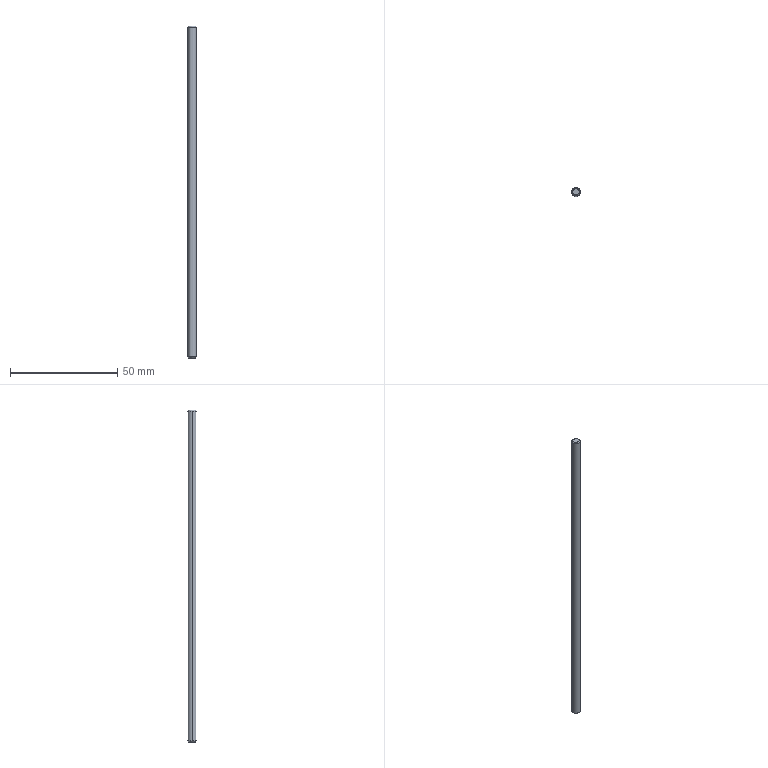Part | STEP file | 11-FG-B01711 | 1 solid | 8 faces | box 4 x 4 x 155 mm | volume 1945 mm3 | cone 4 | cylinder 2 | plane 2 | commonest cylinder face diameters 4 x2
STEP:
#1=CARTESIAN_POINT('',(-1.5,0.,0.));
#2=VERTEX_POINT('',#1);
#3=CARTESIAN_POINT('',(1.5,0.,0.));
#4=VERTEX_POINT('',#3);
#5=CARTESIAN_POINT('',(0.,0.,0.));
#6=DIRECTION('',(0.,0.,-1.));
#7=DIRECTION('',(1.,0.,0.));
#8=AXIS2_PLACEMENT_3D('',#5,#6,#7);
#9=CIRCLE('',#8,1.5);
#10=EDGE_CURVE('',#2,#4,#9,.T.);
#11=ORIENTED_EDGE('',*,*,#10,.F.);
#12=CARTESIAN_POINT('',(-2.,0.,0.5));
#13=VERTEX_POINT('',#12);
#14=CARTESIAN_POINT('',(-2.,0.,0.5));
#15=DIRECTION('',(-0.7071,0.,0.7071));
#16=VECTOR('',#15,1000.);
#17=LINE('',#14,#16);
#18=EDGE_CURVE('',#2,#13,#17,.T.);
#19=ORIENTED_EDGE('',*,*,#18,.T.);
#20=CARTESIAN_POINT('',(2.,0.,0.5));
#21=VERTEX_POINT('',#20);
#22=CARTESIAN_POINT('',(0.,0.,0.5));
#23=DIRECTION('',(0.,0.,1.));
#24=DIRECTION('',(1.,0.,0.));
#25=AXIS2_PLACEMENT_3D('',#22,#23,#24);
#26=CIRCLE('',#25,2.);
#27=EDGE_CURVE('',#21,#13,#26,.T.);
#28=ORIENTED_EDGE('',*,*,#27,.F.);
#29=CARTESIAN_POINT('',(2.,0.,0.5));
#30=DIRECTION('',(0.7071,0.,0.7071));
#31=VECTOR('',#30,1000.);
#32=LINE('',#29,#31);
#33=EDGE_CURVE('',#4,#21,#32,.T.);
#34=ORIENTED_EDGE('',*,*,#33,.F.);
#35=EDGE_LOOP('',(#11,#19,#28,#34));
#36=FACE_OUTER_BOUND('',#35,.T.);
#37=CARTESIAN_POINT('',(0.,0.,0.5));
#38=DIRECTION('',(0.,0.,1.));
#39=DIRECTION('',(1.,0.,0.));
#40=AXIS2_PLACEMENT_3D('',#37,#38,#39);
#41=CONICAL_SURFACE('',#40,2.,0.7854);
#42=ADVANCED_FACE('',(#36),#41,.T.);
#43=CARTESIAN_POINT('',(1.5,0.,155.));
#44=VERTEX_POINT('',#43);
#45=CARTESIAN_POINT('',(-1.5,0.,155.));
#46=VERTEX_POINT('',#45);
#47=CARTESIAN_POINT('',(0.,0.,155.));
#48=DIRECTION('',(0.,0.,1.));
#49=DIRECTION('',(1.,0.,0.));
#50=AXIS2_PLACEMENT_3D('',#47,#48,#49);
#51=CIRCLE('',#50,1.5);
#52=EDGE_CURVE('',#44,#46,#51,.T.);
#53=ORIENTED_EDGE('',*,*,#52,.F.);
#54=CARTESIAN_POINT('',(2.,0.,154.5));
#55=VERTEX_POINT('',#54);
#56=CARTESIAN_POINT('',(1.5,0.,155.));
#57=DIRECTION('',(0.7071,0.,-0.7071));
#58=VECTOR('',#57,1000.);
#59=LINE('',#56,#58);
#60=EDGE_CURVE('',#44,#55,#59,.T.);
#61=ORIENTED_EDGE('',*,*,#60,.T.);
#62=CARTESIAN_POINT('',(-2.,0.,154.5));
#63=VERTEX_POINT('',#62);
#64=CARTESIAN_POINT('',(0.,0.,154.5));
#65=DIRECTION('',(0.,0.,-1.));
#66=DIRECTION('',(1.,0.,0.));
#67=AXIS2_PLACEMENT_3D('',#64,#65,#66);
#68=CIRCLE('',#67,2.);
#69=EDGE_CURVE('',#63,#55,#68,.T.);
#70=ORIENTED_EDGE('',*,*,#69,.F.);
#71=CARTESIAN_POINT('',(-1.5,0.,155.));
#72=DIRECTION('',(-0.7071,0.,-0.7071));
#73=VECTOR('',#72,1000.);
#74=LINE('',#71,#73);
#75=EDGE_CURVE('',#46,#63,#74,.T.);
#76=ORIENTED_EDGE('',*,*,#75,.F.);
#77=EDGE_LOOP('',(#53,#61,#70,#76));
#78=FACE_OUTER_BOUND('',#77,.T.);
#79=CARTESIAN_POINT('',(0.,0.,155.));
#80=DIRECTION('',(0.,0.,-1.));
#81=DIRECTION('',(-1.,0.,0.));
#82=AXIS2_PLACEMENT_3D('',#79,#80,#81);
#83=CONICAL_SURFACE('',#82,1.5,0.7854);
#84=ADVANCED_FACE('',(#78),#83,.T.);
#85=ORIENTED_EDGE('',*,*,#69,.T.);
#86=CARTESIAN_POINT('',(2.,0.,155.));
#87=DIRECTION('',(0.,0.,-1.));
#88=VECTOR('',#87,1000.);
#89=LINE('',#86,#88);
#90=EDGE_CURVE('',#55,#21,#89,.T.);
#91=ORIENTED_EDGE('',*,*,#90,.T.);
#92=ORIENTED_EDGE('',*,*,#27,.T.);
#93=CARTESIAN_POINT('',(-2.,0.,155.));
#94=DIRECTION('',(0.,0.,-1.));
#95=VECTOR('',#94,1000.);
#96=LINE('',#93,#95);
#97=EDGE_CURVE('',#63,#13,#96,.T.);
#98=ORIENTED_EDGE('',*,*,#97,.F.);
#99=EDGE_LOOP('',(#85,#91,#92,#98));
#100=FACE_OUTER_BOUND('',#99,.T.);
#101=CARTESIAN_POINT('',(0.,0.,155.));
#102=DIRECTION('',(0.,0.,-1.));
#103=DIRECTION('',(-1.,0.,0.));
#104=AXIS2_PLACEMENT_3D('',#101,#102,#103);
#105=CYLINDRICAL_SURFACE('',#104,2.);
#106=ADVANCED_FACE('',(#100),#105,.T.);
#107=ORIENTED_EDGE('',*,*,#90,.F.);
#108=CARTESIAN_POINT('',(0.,0.,154.5));
#109=DIRECTION('',(0.,0.,-1.));
#110=DIRECTION('',(1.,0.,0.));
#111=AXIS2_PLACEMENT_3D('',#108,#109,#110);
#112=CIRCLE('',#111,2.);
#113=EDGE_CURVE('',#55,#63,#112,.T.);
#114=ORIENTED_EDGE('',*,*,#113,.T.);
#115=ORIENTED_EDGE('',*,*,#97,.T.);
#116=CARTESIAN_POINT('',(0.,0.,0.5));
#117=DIRECTION('',(0.,0.,1.));
#118=DIRECTION('',(1.,0.,0.));
#119=AXIS2_PLACEMENT_3D('',#116,#117,#118);
#120=CIRCLE('',#119,2.);
#121=EDGE_CURVE('',#13,#21,#120,.T.);
#122=ORIENTED_EDGE('',*,*,#121,.T.);
#123=EDGE_LOOP('',(#107,#114,#115,#122));
#124=FACE_OUTER_BOUND('',#123,.T.);
#125=CARTESIAN_POINT('',(0.,0.,155.));
#126=DIRECTION('',(0.,0.,-1.));
#127=DIRECTION('',(-1.,0.,0.));
#128=AXIS2_PLACEMENT_3D('',#125,#126,#127);
#129=CYLINDRICAL_SURFACE('',#128,2.);
#130=ADVANCED_FACE('',(#124),#129,.T.);
#131=CARTESIAN_POINT('',(0.,0.,155.));
#132=DIRECTION('',(0.,0.,1.));
#133=DIRECTION('',(1.,0.,0.));
#134=AXIS2_PLACEMENT_3D('',#131,#132,#133);
#135=CIRCLE('',#134,1.5);
#136=EDGE_CURVE('',#46,#44,#135,.T.);
#137=ORIENTED_EDGE('',*,*,#136,.T.);
#138=ORIENTED_EDGE('',*,*,#52,.T.);
#139=EDGE_LOOP('',(#137,#138));
#140=FACE_OUTER_BOUND('',#139,.T.);
#141=CARTESIAN_POINT('',(0.,0.,155.));
#142=DIRECTION('',(0.,0.,1.));
#143=DIRECTION('',(1.,0.,0.));
#144=AXIS2_PLACEMENT_3D('',#141,#142,#143);
#145=PLANE('',#144);
#146=ADVANCED_FACE('',(#140),#145,.T.);
#147=CARTESIAN_POINT('',(0.,0.,0.));
#148=DIRECTION('',(0.,0.,-1.));
#149=DIRECTION('',(1.,0.,0.));
#150=AXIS2_PLACEMENT_3D('',#147,#148,#149);
#151=CIRCLE('',#150,1.5);
#152=EDGE_CURVE('',#4,#2,#151,.T.);
#153=ORIENTED_EDGE('',*,*,#152,.T.);
#154=ORIENTED_EDGE('',*,*,#10,.T.);
#155=EDGE_LOOP('',(#153,#154));
#156=FACE_OUTER_BOUND('',#155,.T.);
#157=CARTESIAN_POINT('',(0.,0.,0.));
#158=DIRECTION('',(0.,0.,1.));
#159=DIRECTION('',(1.,0.,0.));
#160=AXIS2_PLACEMENT_3D('',#157,#158,#159);
#161=PLANE('',#160);
#162=ADVANCED_FACE('',(#156),#161,.F.);
#163=ORIENTED_EDGE('',*,*,#60,.F.);
#164=ORIENTED_EDGE('',*,*,#136,.F.);
#165=ORIENTED_EDGE('',*,*,#75,.T.);
#166=ORIENTED_EDGE('',*,*,#113,.F.);
#167=EDGE_LOOP('',(#163,#164,#165,#166));
#168=FACE_OUTER_BOUND('',#167,.T.);
#169=CARTESIAN_POINT('',(0.,0.,155.));
#170=DIRECTION('',(0.,0.,-1.));
#171=DIRECTION('',(-1.,0.,0.));
#172=AXIS2_PLACEMENT_3D('',#169,#170,#171);
#173=CONICAL_SURFACE('',#172,1.5,0.7854);
#174=ADVANCED_FACE('',(#168),#173,.T.);
#175=ORIENTED_EDGE('',*,*,#18,.F.);
#176=ORIENTED_EDGE('',*,*,#152,.F.);
#177=ORIENTED_EDGE('',*,*,#33,.T.);
#178=ORIENTED_EDGE('',*,*,#121,.F.);
#179=EDGE_LOOP('',(#175,#176,#177,#178));
#180=FACE_OUTER_BOUND('',#179,.T.);
#181=CARTESIAN_POINT('',(0.,0.,0.5));
#182=DIRECTION('',(0.,0.,1.));
#183=DIRECTION('',(1.,0.,0.));
#184=AXIS2_PLACEMENT_3D('',#181,#182,#183);
#185=CONICAL_SURFACE('',#184,2.,0.7854);
#186=ADVANCED_FACE('',(#180),#185,.T.);
#187=CLOSED_SHELL('',(#42,#84,#106,#130,#146,#162,#174,#186));
#188=MANIFOLD_SOLID_BREP('',#187);
#189=CARTESIAN_POINT('',(0.,0.,0.));
#190=DIRECTION('',(0.,0.,1.));
#191=DIRECTION('',(1.,0.,0.));
#192=AXIS2_PLACEMENT_3D('',#189,#190,#191);
#193=(LENGTH_UNIT()NAMED_UNIT(*)SI_UNIT(.MILLI.,.METRE.));
#194=UNCERTAINTY_MEASURE_WITH_UNIT(LENGTH_MEASURE(0.00001),#193,'','');
#195=(NAMED_UNIT(*)PLANE_ANGLE_UNIT()SI_UNIT($,.RADIAN.));
#196=(NAMED_UNIT(*)SI_UNIT($,.STERADIAN.)SOLID_ANGLE_UNIT());
#197=(GEOMETRIC_REPRESENTATION_CONTEXT(3)GLOBAL_UNCERTAINTY_ASSIGNED_CONTEXT((#194))GLOBAL_UNIT_ASSIGNED_CONTEXT((#193,#195,#196))REPRESENTATION_CONTEXT('',''));
#198=ADVANCED_BREP_SHAPE_REPRESENTATION('',(#188,#192),#197);